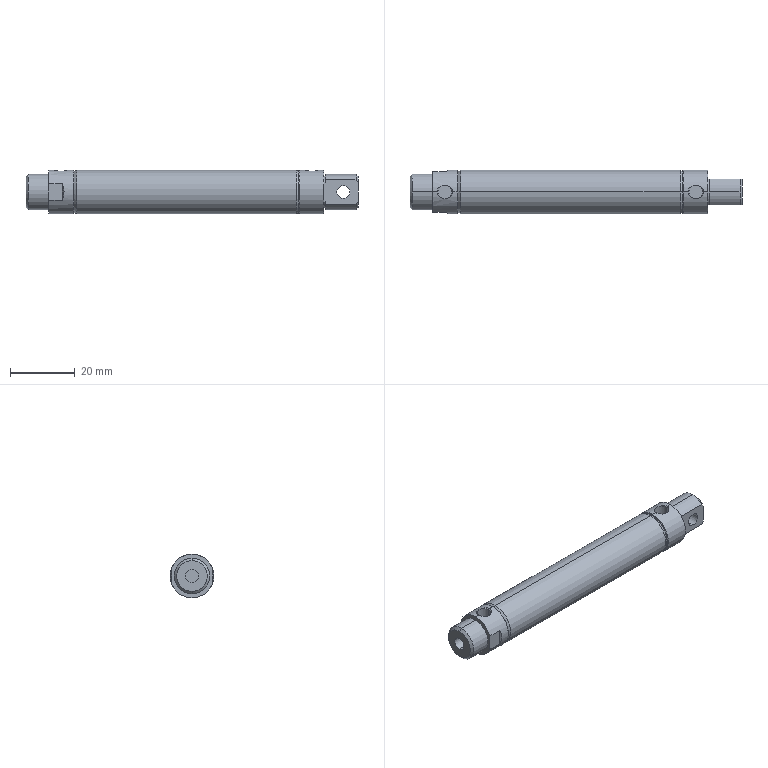Part | SolidWorks | features RefAxis 18, 3DProfileFeature 6, ICE 4, RevCut 2, Revolution 1, Scale 1 | 1 solid | 61 faces | box 102.5 x 13.5 x 13.5 mm | volume 7743 mm3 | cylinder 24 | cone 19 | plane 18 | commonest cylinder face diameters 13.5 x6 10 x5 11 x5 4 x4 4.283 x4